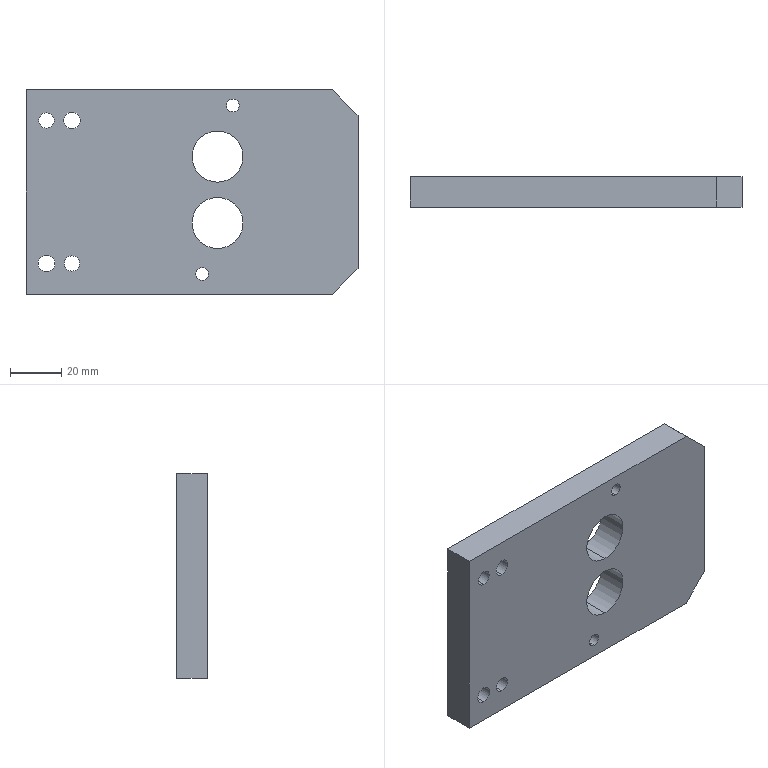Part | SolidWorks | features HoleWzd 3, 3DProfileFeature 2, Chamfer 1, Extrusion 1, ICE 1 | 1 solid | 30 faces | box 130 x 12 x 80 mm | volume 113262 mm3 | cylinder 20 | plane 10 | commonest cylinder face diameters 5 x4 6 x4 6.6 x4 11 x4 20 x4
STEP:
#1=CARTESIAN_POINT('',(81.,0.,-8.642));
#2=VERTEX_POINT('',#1);
#3=CARTESIAN_POINT('',(81.,0.,-3.642));
#4=VERTEX_POINT('',#3);
#5=CARTESIAN_POINT('',(81.,0.,-6.142));
#6=DIRECTION('',(0.,1.,0.));
#7=DIRECTION('',(0.,0.,1.));
#8=AXIS2_PLACEMENT_3D('',#5,#6,#7);
#9=CIRCLE('',#8,2.5);
#10=EDGE_CURVE('',#2,#4,#9,.T.);
#11=ORIENTED_EDGE('',*,*,#10,.F.);
#12=CARTESIAN_POINT('',(81.,12.,-8.642));
#13=VERTEX_POINT('',#12);
#14=CARTESIAN_POINT('',(81.,0.,-8.642));
#15=DIRECTION('',(0.,1.,0.));
#16=VECTOR('',#15,1000.);
#17=LINE('',#14,#16);
#18=EDGE_CURVE('',#2,#13,#17,.T.);
#19=ORIENTED_EDGE('',*,*,#18,.T.);
#20=CARTESIAN_POINT('',(81.,12.,-3.642));
#21=VERTEX_POINT('',#20);
#22=CARTESIAN_POINT('',(81.,12.,-6.142));
#23=DIRECTION('',(0.,1.,0.));
#24=DIRECTION('',(0.,0.,1.));
#25=AXIS2_PLACEMENT_3D('',#22,#23,#24);
#26=CIRCLE('',#25,2.5);
#27=EDGE_CURVE('',#13,#21,#26,.T.);
#28=ORIENTED_EDGE('',*,*,#27,.T.);
#29=CARTESIAN_POINT('',(81.,0.,-3.642));
#30=DIRECTION('',(0.,1.,0.));
#31=VECTOR('',#30,1000.);
#32=LINE('',#29,#31);
#33=EDGE_CURVE('',#4,#21,#32,.T.);
#34=ORIENTED_EDGE('',*,*,#33,.F.);
#35=EDGE_LOOP('',(#11,#19,#28,#34));
#36=FACE_OUTER_BOUND('',#35,.T.);
#37=CARTESIAN_POINT('',(81.,0.,-6.142));
#38=DIRECTION('',(0.,1.,0.));
#39=DIRECTION('',(0.,0.,1.));
#40=AXIS2_PLACEMENT_3D('',#37,#38,#39);
#41=CYLINDRICAL_SURFACE('',#40,2.5);
#42=ADVANCED_FACE('',(#36),#41,.F.);
#43=CARTESIAN_POINT('',(69.,0.,-74.642));
#44=VERTEX_POINT('',#43);
#45=CARTESIAN_POINT('',(69.,0.,-69.642));
#46=VERTEX_POINT('',#45);
#47=CARTESIAN_POINT('',(69.,0.,-72.142));
#48=DIRECTION('',(0.,1.,0.));
#49=DIRECTION('',(0.,0.,1.));
#50=AXIS2_PLACEMENT_3D('',#47,#48,#49);
#51=CIRCLE('',#50,2.5);
#52=EDGE_CURVE('',#44,#46,#51,.T.);
#53=ORIENTED_EDGE('',*,*,#52,.F.);
#54=CARTESIAN_POINT('',(69.,12.,-74.642));
#55=VERTEX_POINT('',#54);
#56=CARTESIAN_POINT('',(69.,0.,-74.642));
#57=DIRECTION('',(0.,1.,0.));
#58=VECTOR('',#57,1000.);
#59=LINE('',#56,#58);
#60=EDGE_CURVE('',#44,#55,#59,.T.);
#61=ORIENTED_EDGE('',*,*,#60,.T.);
#62=CARTESIAN_POINT('',(69.,12.,-69.642));
#63=VERTEX_POINT('',#62);
#64=CARTESIAN_POINT('',(69.,12.,-72.142));
#65=DIRECTION('',(0.,1.,0.));
#66=DIRECTION('',(0.,0.,1.));
#67=AXIS2_PLACEMENT_3D('',#64,#65,#66);
#68=CIRCLE('',#67,2.5);
#69=EDGE_CURVE('',#55,#63,#68,.T.);
#70=ORIENTED_EDGE('',*,*,#69,.T.);
#71=CARTESIAN_POINT('',(69.,0.,-69.642));
#72=DIRECTION('',(0.,1.,0.));
#73=VECTOR('',#72,1000.);
#74=LINE('',#71,#73);
#75=EDGE_CURVE('',#46,#63,#74,.T.);
#76=ORIENTED_EDGE('',*,*,#75,.F.);
#77=EDGE_LOOP('',(#53,#61,#70,#76));
#78=FACE_OUTER_BOUND('',#77,.T.);
#79=CARTESIAN_POINT('',(69.,0.,-72.142));
#80=DIRECTION('',(0.,1.,0.));
#81=DIRECTION('',(0.,0.,1.));
#82=AXIS2_PLACEMENT_3D('',#79,#80,#81);
#83=CYLINDRICAL_SURFACE('',#82,2.5);
#84=ADVANCED_FACE('',(#78),#83,.F.);
#85=CARTESIAN_POINT('',(75.,12.,-42.142));
#86=VERTEX_POINT('',#85);
#87=CARTESIAN_POINT('',(75.,12.,-62.142));
#88=VERTEX_POINT('',#87);
#89=CARTESIAN_POINT('',(75.,12.,-52.142));
#90=DIRECTION('',(0.,-1.,0.));
#91=DIRECTION('',(0.,0.,-1.));
#92=AXIS2_PLACEMENT_3D('',#89,#90,#91);
#93=CIRCLE('',#92,10.);
#94=EDGE_CURVE('',#86,#88,#93,.T.);
#95=ORIENTED_EDGE('',*,*,#94,.F.);
#96=CARTESIAN_POINT('',(75.,0.,-42.142));
#97=VERTEX_POINT('',#96);
#98=CARTESIAN_POINT('',(75.,0.,-42.142));
#99=DIRECTION('',(0.,-1.,0.));
#100=VECTOR('',#99,1000.);
#101=LINE('',#98,#100);
#102=EDGE_CURVE('',#86,#97,#101,.T.);
#103=ORIENTED_EDGE('',*,*,#102,.T.);
#104=CARTESIAN_POINT('',(75.,0.,-62.142));
#105=VERTEX_POINT('',#104);
#106=CARTESIAN_POINT('',(75.,0.,-52.142));
#107=DIRECTION('',(0.,-1.,0.));
#108=DIRECTION('',(0.,0.,-1.));
#109=AXIS2_PLACEMENT_3D('',#106,#107,#108);
#110=CIRCLE('',#109,10.);
#111=EDGE_CURVE('',#97,#105,#110,.T.);
#112=ORIENTED_EDGE('',*,*,#111,.T.);
#113=CARTESIAN_POINT('',(75.,0.,-62.142));
#114=DIRECTION('',(0.,-1.,0.));
#115=VECTOR('',#114,1000.);
#116=LINE('',#113,#115);
#117=EDGE_CURVE('',#88,#105,#116,.T.);
#118=ORIENTED_EDGE('',*,*,#117,.F.);
#119=EDGE_LOOP('',(#95,#103,#112,#118));
#120=FACE_OUTER_BOUND('',#119,.T.);
#121=CARTESIAN_POINT('',(75.,0.,-52.142));
#122=DIRECTION('',(0.,-1.,0.));
#123=DIRECTION('',(0.,0.,-1.));
#124=AXIS2_PLACEMENT_3D('',#121,#122,#123);
#125=CYLINDRICAL_SURFACE('',#124,10.);
#126=ADVANCED_FACE('',(#120),#125,.F.);
#127=CARTESIAN_POINT('',(75.,12.,-16.142));
#128=VERTEX_POINT('',#127);
#129=CARTESIAN_POINT('',(75.,12.,-36.142));
#130=VERTEX_POINT('',#129);
#131=CARTESIAN_POINT('',(75.,12.,-26.142));
#132=DIRECTION('',(0.,-1.,0.));
#133=DIRECTION('',(0.,0.,-1.));
#134=AXIS2_PLACEMENT_3D('',#131,#132,#133);
#135=CIRCLE('',#134,10.);
#136=EDGE_CURVE('',#128,#130,#135,.T.);
#137=ORIENTED_EDGE('',*,*,#136,.F.);
#138=CARTESIAN_POINT('',(75.,0.,-16.142));
#139=VERTEX_POINT('',#138);
#140=CARTESIAN_POINT('',(75.,0.,-16.142));
#141=DIRECTION('',(0.,-1.,0.));
#142=VECTOR('',#141,1000.);
#143=LINE('',#140,#142);
#144=EDGE_CURVE('',#128,#139,#143,.T.);
#145=ORIENTED_EDGE('',*,*,#144,.T.);
#146=CARTESIAN_POINT('',(75.,0.,-36.142));
#147=VERTEX_POINT('',#146);
#148=CARTESIAN_POINT('',(75.,0.,-26.142));
#149=DIRECTION('',(0.,-1.,0.));
#150=DIRECTION('',(0.,0.,-1.));
#151=AXIS2_PLACEMENT_3D('',#148,#149,#150);
#152=CIRCLE('',#151,10.);
#153=EDGE_CURVE('',#139,#147,#152,.T.);
#154=ORIENTED_EDGE('',*,*,#153,.T.);
#155=CARTESIAN_POINT('',(75.,0.,-36.142));
#156=DIRECTION('',(0.,-1.,0.));
#157=VECTOR('',#156,1000.);
#158=LINE('',#155,#157);
#159=EDGE_CURVE('',#130,#147,#158,.T.);
#160=ORIENTED_EDGE('',*,*,#159,.F.);
#161=EDGE_LOOP('',(#137,#145,#154,#160));
#162=FACE_OUTER_BOUND('',#161,.T.);
#163=CARTESIAN_POINT('',(75.,0.,-26.142));
#164=DIRECTION('',(0.,-1.,0.));
#165=DIRECTION('',(0.,0.,-1.));
#166=AXIS2_PLACEMENT_3D('',#163,#164,#165);
#167=CYLINDRICAL_SURFACE('',#166,10.);
#168=ADVANCED_FACE('',(#162),#167,.F.);
#169=CARTESIAN_POINT('',(18.,0.,-71.));
#170=VERTEX_POINT('',#169);
#171=CARTESIAN_POINT('',(18.,0.,-65.));
#172=VERTEX_POINT('',#171);
#173=CARTESIAN_POINT('',(18.,0.,-68.));
#174=DIRECTION('',(0.,1.,0.));
#175=DIRECTION('',(0.,0.,1.));
#176=AXIS2_PLACEMENT_3D('',#173,#174,#175);
#177=CIRCLE('',#176,3.);
#178=EDGE_CURVE('',#170,#172,#177,.T.);
#179=ORIENTED_EDGE('',*,*,#178,.F.);
#180=CARTESIAN_POINT('',(18.,12.,-71.));
#181=VERTEX_POINT('',#180);
#182=CARTESIAN_POINT('',(18.,12.,-71.));
#183=DIRECTION('',(0.,1.,0.));
#184=VECTOR('',#183,1000.);
#185=LINE('',#182,#184);
#186=EDGE_CURVE('',#170,#181,#185,.T.);
#187=ORIENTED_EDGE('',*,*,#186,.T.);
#188=CARTESIAN_POINT('',(18.,12.,-65.));
#189=VERTEX_POINT('',#188);
#190=CARTESIAN_POINT('',(18.,12.,-68.));
#191=DIRECTION('',(0.,1.,0.));
#192=DIRECTION('',(0.,0.,1.));
#193=AXIS2_PLACEMENT_3D('',#190,#191,#192);
#194=CIRCLE('',#193,3.);
#195=EDGE_CURVE('',#181,#189,#194,.T.);
#196=ORIENTED_EDGE('',*,*,#195,.T.);
#197=CARTESIAN_POINT('',(18.,12.,-65.));
#198=DIRECTION('',(0.,1.,0.));
#199=VECTOR('',#198,1000.);
#200=LINE('',#197,#199);
#201=EDGE_CURVE('',#172,#189,#200,.T.);
#202=ORIENTED_EDGE('',*,*,#201,.F.);
#203=EDGE_LOOP('',(#179,#187,#196,#202));
#204=FACE_OUTER_BOUND('',#203,.T.);
#205=CARTESIAN_POINT('',(18.,12.,-68.));
#206=DIRECTION('',(0.,1.,0.));
#207=DIRECTION('',(0.,0.,1.));
#208=AXIS2_PLACEMENT_3D('',#205,#206,#207);
#209=CYLINDRICAL_SURFACE('',#208,3.);
#210=ADVANCED_FACE('',(#204),#209,.F.);
#211=CARTESIAN_POINT('',(8.,0.,-15.));
#212=VERTEX_POINT('',#211);
#213=CARTESIAN_POINT('',(8.,0.,-9.));
#214=VERTEX_POINT('',#213);
#215=CARTESIAN_POINT('',(8.,0.,-12.));
#216=DIRECTION('',(0.,1.,0.));
#217=DIRECTION('',(0.,0.,1.));
#218=AXIS2_PLACEMENT_3D('',#215,#216,#217);
#219=CIRCLE('',#218,3.);
#220=EDGE_CURVE('',#212,#214,#219,.T.);
#221=ORIENTED_EDGE('',*,*,#220,.F.);
#222=CARTESIAN_POINT('',(8.,12.,-15.));
#223=VERTEX_POINT('',#222);
#224=CARTESIAN_POINT('',(8.,12.,-15.));
#225=DIRECTION('',(0.,1.,0.));
#226=VECTOR('',#225,1000.);
#227=LINE('',#224,#226);
#228=EDGE_CURVE('',#212,#223,#227,.T.);
#229=ORIENTED_EDGE('',*,*,#228,.T.);
#230=CARTESIAN_POINT('',(8.,12.,-9.));
#231=VERTEX_POINT('',#230);
#232=CARTESIAN_POINT('',(8.,12.,-12.));
#233=DIRECTION('',(0.,1.,0.));
#234=DIRECTION('',(0.,0.,1.));
#235=AXIS2_PLACEMENT_3D('',#232,#233,#234);
#236=CIRCLE('',#235,3.);
#237=EDGE_CURVE('',#223,#231,#236,.T.);
#238=ORIENTED_EDGE('',*,*,#237,.T.);
#239=CARTESIAN_POINT('',(8.,12.,-9.));
#240=DIRECTION('',(0.,1.,0.));
#241=VECTOR('',#240,1000.);
#242=LINE('',#239,#241);
#243=EDGE_CURVE('',#214,#231,#242,.T.);
#244=ORIENTED_EDGE('',*,*,#243,.F.);
#245=EDGE_LOOP('',(#221,#229,#238,#244));
#246=FACE_OUTER_BOUND('',#245,.T.);
#247=CARTESIAN_POINT('',(8.,12.,-12.));
#248=DIRECTION('',(0.,1.,0.));
#249=DIRECTION('',(0.,0.,1.));
#250=AXIS2_PLACEMENT_3D('',#247,#248,#249);
#251=CYLINDRICAL_SURFACE('',#250,3.);
#252=ADVANCED_FACE('',(#246),#251,.F.);
#253=CARTESIAN_POINT('',(8.,5.2,-73.5));
#254=VERTEX_POINT('',#253);
#255=CARTESIAN_POINT('',(8.,5.2,-62.5));
#256=VERTEX_POINT('',#255);
#257=CARTESIAN_POINT('',(8.,5.2,-68.));
#258=DIRECTION('',(0.,1.,0.));
#259=DIRECTION('',(0.,0.,1.));
#260=AXIS2_PLACEMENT_3D('',#257,#258,#259);
#261=CIRCLE('',#260,5.5);
#262=EDGE_CURVE('',#254,#256,#261,.T.);
#263=ORIENTED_EDGE('',*,*,#262,.F.);
#264=CARTESIAN_POINT('',(8.,12.,-73.5));
#265=VERTEX_POINT('',#264);
#266=CARTESIAN_POINT('',(8.,12.,-73.5));
#267=DIRECTION('',(0.,1.,0.));
#268=VECTOR('',#267,1000.);
#269=LINE('',#266,#268);
#270=EDGE_CURVE('',#254,#265,#269,.T.);
#271=ORIENTED_EDGE('',*,*,#270,.T.);
#272=CARTESIAN_POINT('',(8.,12.,-62.5));
#273=VERTEX_POINT('',#272);
#274=CARTESIAN_POINT('',(8.,12.,-68.));
#275=DIRECTION('',(0.,1.,0.));
#276=DIRECTION('',(0.,0.,1.));
#277=AXIS2_PLACEMENT_3D('',#274,#275,#276);
#278=CIRCLE('',#277,5.5);
#279=EDGE_CURVE('',#265,#273,#278,.T.);
#280=ORIENTED_EDGE('',*,*,#279,.T.);
#281=CARTESIAN_POINT('',(8.,12.,-62.5));
#282=DIRECTION('',(0.,1.,0.));
#283=VECTOR('',#282,1000.);
#284=LINE('',#281,#283);
#285=EDGE_CURVE('',#256,#273,#284,.T.);
#286=ORIENTED_EDGE('',*,*,#285,.F.);
#287=EDGE_LOOP('',(#263,#271,#280,#286));
#288=FACE_OUTER_BOUND('',#287,.T.);
#289=CARTESIAN_POINT('',(8.,12.,-68.));
#290=DIRECTION('',(0.,1.,0.));
#291=DIRECTION('',(0.,0.,1.));
#292=AXIS2_PLACEMENT_3D('',#289,#290,#291);
#293=CYLINDRICAL_SURFACE('',#292,5.5);
#294=ADVANCED_FACE('',(#288),#293,.F.);
#295=CARTESIAN_POINT('',(8.,0.,-71.3));
#296=VERTEX_POINT('',#295);
#297=CARTESIAN_POINT('',(8.,0.,-64.7));
#298=VERTEX_POINT('',#297);
#299=CARTESIAN_POINT('',(8.,0.,-68.));
#300=DIRECTION('',(0.,1.,0.));
#301=DIRECTION('',(0.,0.,1.));
#302=AXIS2_PLACEMENT_3D('',#299,#300,#301);
#303=CIRCLE('',#302,3.3);
#304=EDGE_CURVE('',#296,#298,#303,.T.);
#305=ORIENTED_EDGE('',*,*,#304,.F.);
#306=CARTESIAN_POINT('',(8.,5.2,-71.3));
#307=VERTEX_POINT('',#306);
#308=CARTESIAN_POINT('',(8.,12.,-71.3));
#309=DIRECTION('',(0.,1.,0.));
#310=VECTOR('',#309,1000.);
#311=LINE('',#308,#310);
#312=EDGE_CURVE('',#296,#307,#311,.T.);
#313=ORIENTED_EDGE('',*,*,#312,.T.);
#314=CARTESIAN_POINT('',(8.,5.2,-64.7));
#315=VERTEX_POINT('',#314);
#316=CARTESIAN_POINT('',(8.,5.2,-68.));
#317=DIRECTION('',(0.,1.,0.));
#318=DIRECTION('',(0.,0.,1.));
#319=AXIS2_PLACEMENT_3D('',#316,#317,#318);
#320=CIRCLE('',#319,3.3);
#321=EDGE_CURVE('',#307,#315,#320,.T.);
#322=ORIENTED_EDGE('',*,*,#321,.T.);
#323=CARTESIAN_POINT('',(8.,12.,-64.7));
#324=DIRECTION('',(0.,1.,0.));
#325=VECTOR('',#324,1000.);
#326=LINE('',#323,#325);
#327=EDGE_CURVE('',#298,#315,#326,.T.);
#328=ORIENTED_EDGE('',*,*,#327,.F.);
#329=EDGE_LOOP('',(#305,#313,#322,#328));
#330=FACE_OUTER_BOUND('',#329,.T.);
#331=CARTESIAN_POINT('',(8.,12.,-68.));
#332=DIRECTION('',(0.,1.,0.));
#333=DIRECTION('',(0.,0.,1.));
#334=AXIS2_PLACEMENT_3D('',#331,#332,#333);
#335=CYLINDRICAL_SURFACE('',#334,3.3);
#336=ADVANCED_FACE('',(#330),#335,.F.);
#337=CARTESIAN_POINT('',(18.,5.2,-17.5));
#338=VERTEX_POINT('',#337);
#339=CARTESIAN_POINT('',(18.,5.2,-6.5));
#340=VERTEX_POINT('',#339);
#341=CARTESIAN_POINT('',(18.,5.2,-12.));
#342=DIRECTION('',(0.,1.,0.));
#343=DIRECTION('',(0.,0.,1.));
#344=AXIS2_PLACEMENT_3D('',#341,#342,#343);
#345=CIRCLE('',#344,5.5);
#346=EDGE_CURVE('',#338,#340,#345,.T.);
#347=ORIENTED_EDGE('',*,*,#346,.F.);
#348=CARTESIAN_POINT('',(18.,12.,-17.5));
#349=VERTEX_POINT('',#348);
#350=CARTESIAN_POINT('',(18.,12.,-17.5));
#351=DIRECTION('',(0.,1.,0.));
#352=VECTOR('',#351,1000.);
#353=LINE('',#350,#352);
#354=EDGE_CURVE('',#338,#349,#353,.T.);
#355=ORIENTED_EDGE('',*,*,#354,.T.);
#356=CARTESIAN_POINT('',(18.,12.,-6.5));
#357=VERTEX_POINT('',#356);
#358=CARTESIAN_POINT('',(18.,12.,-12.));
#359=DIRECTION('',(0.,1.,0.));
#360=DIRECTION('',(0.,0.,1.));
#361=AXIS2_PLACEMENT_3D('',#358,#359,#360);
#362=CIRCLE('',#361,5.5);
#363=EDGE_CURVE('',#349,#357,#362,.T.);
#364=ORIENTED_EDGE('',*,*,#363,.T.);
#365=CARTESIAN_POINT('',(18.,12.,-6.5));
#366=DIRECTION('',(0.,1.,0.));
#367=VECTOR('',#366,1000.);
#368=LINE('',#365,#367);
#369=EDGE_CURVE('',#340,#357,#368,.T.);
#370=ORIENTED_EDGE('',*,*,#369,.F.);
#371=EDGE_LOOP('',(#347,#355,#364,#370));
#372=FACE_OUTER_BOUND('',#371,.T.);
#373=CARTESIAN_POINT('',(18.,12.,-12.));
#374=DIRECTION('',(0.,1.,0.));
#375=DIRECTION('',(0.,0.,1.));
#376=AXIS2_PLACEMENT_3D('',#373,#374,#375);
#377=CYLINDRICAL_SURFACE('',#376,5.5);
#378=ADVANCED_FACE('',(#372),#377,.F.);
#379=CARTESIAN_POINT('',(18.,0.,-15.3));
#380=VERTEX_POINT('',#379);
#381=CARTESIAN_POINT('',(18.,0.,-8.7));
#382=VERTEX_POINT('',#381);
#383=CARTESIAN_POINT('',(18.,0.,-12.));
#384=DIRECTION('',(0.,1.,0.));
#385=DIRECTION('',(0.,0.,1.));
#386=AXIS2_PLACEMENT_3D('',#383,#384,#385);
#387=CIRCLE('',#386,3.3);
#388=EDGE_CURVE('',#380,#382,#387,.T.);
#389=ORIENTED_EDGE('',*,*,#388,.F.);
#390=CARTESIAN_POINT('',(18.,5.2,-15.3));
#391=VERTEX_POINT('',#390);
#392=CARTESIAN_POINT('',(18.,12.,-15.3));
#393=DIRECTION('',(0.,1.,0.));
#394=VECTOR('',#393,1000.);
#395=LINE('',#392,#394);
#396=EDGE_CURVE('',#380,#391,#395,.T.);
#397=ORIENTED_EDGE('',*,*,#396,.T.);
#398=CARTESIAN_POINT('',(18.,5.2,-8.7));
#399=VERTEX_POINT('',#398);
#400=CARTESIAN_POINT('',(18.,5.2,-12.));
#401=DIRECTION('',(0.,1.,0.));
#402=DIRECTION('',(0.,0.,1.));
#403=AXIS2_PLACEMENT_3D('',#400,#401,#402);
#404=CIRCLE('',#403,3.3);
#405=EDGE_CURVE('',#391,#399,#404,.T.);
#406=ORIENTED_EDGE('',*,*,#405,.T.);
#407=CARTESIAN_POINT('',(18.,12.,-8.7));
#408=DIRECTION('',(0.,1.,0.));
#409=VECTOR('',#408,1000.);
#410=LINE('',#407,#409);
#411=EDGE_CURVE('',#382,#399,#410,.T.);
#412=ORIENTED_EDGE('',*,*,#411,.F.);
#413=EDGE_LOOP('',(#389,#397,#406,#412));
#414=FACE_OUTER_BOUND('',#413,.T.);
#415=CARTESIAN_POINT('',(18.,12.,-12.));
#416=DIRECTION('',(0.,1.,0.));
#417=DIRECTION('',(0.,0.,1.));
#418=AXIS2_PLACEMENT_3D('',#415,#416,#417);
#419=CYLINDRICAL_SURFACE('',#418,3.3);
#420=ADVANCED_FACE('',(#414),#419,.F.);
#421=CARTESIAN_POINT('',(81.,0.,-6.142));
#422=DIRECTION('',(0.,1.,0.));
#423=DIRECTION('',(0.,0.,1.));
#424=AXIS2_PLACEMENT_3D('',#421,#422,#423);
#425=CIRCLE('',#424,2.5);
#426=EDGE_CURVE('',#4,#2,#425,.T.);
#427=ORIENTED_EDGE('',*,*,#426,.T.);
#428=ORIENTED_EDGE('',*,*,#10,.T.);
#429=EDGE_LOOP('',(#427,#428));
#430=FACE_BOUND('',#429,.T.);
#431=CARTESIAN_POINT('',(69.,0.,-72.142));
#432=DIRECTION('',(0.,1.,0.));
#433=DIRECTION('',(0.,0.,1.));
#434=AXIS2_PLACEMENT_3D('',#431,#432,#433);
#435=CIRCLE('',#434,2.5);
#436=EDGE_CURVE('',#46,#44,#435,.T.);
#437=ORIENTED_EDGE('',*,*,#436,.T.);
#438=ORIENTED_EDGE('',*,*,#52,.T.);
#439=EDGE_LOOP('',(#437,#438));
#440=FACE_BOUND('',#439,.T.);
#441=CARTESIAN_POINT('',(75.,0.,-52.142));
#442=DIRECTION('',(0.,-1.,0.));
#443=DIRECTION('',(0.,0.,-1.));
#444=AXIS2_PLACEMENT_3D('',#441,#442,#443);
#445=CIRCLE('',#444,10.);
#446=EDGE_CURVE('',#105,#97,#445,.T.);
#447=ORIENTED_EDGE('',*,*,#446,.F.);
#448=ORIENTED_EDGE('',*,*,#111,.F.);
#449=EDGE_LOOP('',(#447,#448));
#450=FACE_BOUND('',#449,.T.);
#451=CARTESIAN_POINT('',(75.,0.,-26.142));
#452=DIRECTION('',(0.,-1.,0.));
#453=DIRECTION('',(0.,0.,-1.));
#454=AXIS2_PLACEMENT_3D('',#451,#452,#453);
#455=CIRCLE('',#454,10.);
#456=EDGE_CURVE('',#147,#139,#455,.T.);
#457=ORIENTED_EDGE('',*,*,#456,.F.);
#458=ORIENTED_EDGE('',*,*,#153,.F.);
#459=EDGE_LOOP('',(#457,#458));
#460=FACE_BOUND('',#459,.T.);
#461=CARTESIAN_POINT('',(18.,0.,-68.));
#462=DIRECTION('',(0.,1.,0.));
#463=DIRECTION('',(0.,0.,1.));
#464=AXIS2_PLACEMENT_3D('',#461,#462,#463);
#465=CIRCLE('',#464,3.);
#466=EDGE_CURVE('',#172,#170,#465,.T.);
#467=ORIENTED_EDGE('',*,*,#466,.T.);
#468=ORIENTED_EDGE('',*,*,#178,.T.);
#469=EDGE_LOOP('',(#467,#468));
#470=FACE_BOUND('',#469,.T.);
#471=CARTESIAN_POINT('',(120.,0.,-80.));
#472=VERTEX_POINT('',#471);
#473=CARTESIAN_POINT('',(0.,0.,-80.));
#474=VERTEX_POINT('',#473);
#475=CARTESIAN_POINT('',(0.,0.,-80.));
#476=DIRECTION('',(-1.,0.,0.));
#477=VECTOR('',#476,1000.);
#478=LINE('',#475,#477);
#479=EDGE_CURVE('',#472,#474,#478,.T.);
#480=ORIENTED_EDGE('',*,*,#479,.F.);
#481=CARTESIAN_POINT('',(130.,0.,-70.));
#482=VERTEX_POINT('',#481);
#483=CARTESIAN_POINT('',(100.,0.,-100.));
#484=DIRECTION('',(0.7071,0.,0.7071));
#485=VECTOR('',#484,1000.);
#486=LINE('',#483,#485);
#487=EDGE_CURVE('',#472,#482,#486,.T.);
#488=ORIENTED_EDGE('',*,*,#487,.T.);
#489=CARTESIAN_POINT('',(130.,0.,-10.));
#490=VERTEX_POINT('',#489);
#491=CARTESIAN_POINT('',(130.,0.,0.));
#492=DIRECTION('',(0.,0.,-1.));
#493=VECTOR('',#492,1000.);
#494=LINE('',#491,#493);
#495=EDGE_CURVE('',#490,#482,#494,.T.);
#496=ORIENTED_EDGE('',*,*,#495,.F.);
#497=CARTESIAN_POINT('',(120.,0.,0.));
#498=VERTEX_POINT('',#497);
#499=CARTESIAN_POINT('',(60.,0.,60.));
#500=DIRECTION('',(-0.7071,0.,0.7071));
#501=VECTOR('',#500,1000.);
#502=LINE('',#499,#501);
#503=EDGE_CURVE('',#490,#498,#502,.T.);
#504=ORIENTED_EDGE('',*,*,#503,.T.);
#505=CARTESIAN_POINT('',(0.,0.,0.));
#506=VERTEX_POINT('',#505);
#507=CARTESIAN_POINT('',(0.,0.,0.));
#508=DIRECTION('',(1.,0.,0.));
#509=VECTOR('',#508,1000.);
#510=LINE('',#507,#509);
#511=EDGE_CURVE('',#506,#498,#510,.T.);
#512=ORIENTED_EDGE('',*,*,#511,.F.);
#513=CARTESIAN_POINT('',(0.,0.,0.));
#514=DIRECTION('',(0.,0.,1.));
#515=VECTOR('',#514,1000.);
#516=LINE('',#513,#515);
#517=EDGE_CURVE('',#474,#506,#516,.T.);
#518=ORIENTED_EDGE('',*,*,#517,.F.);
#519=EDGE_LOOP('',(#480,#488,#496,#504,#512,#518));
#520=FACE_OUTER_BOUND('',#519,.T.);
#521=CARTESIAN_POINT('',(18.,0.,-12.));
#522=DIRECTION('',(0.,1.,0.));
#523=DIRECTION('',(0.,0.,1.));
#524=AXIS2_PLACEMENT_3D('',#521,#522,#523);
#525=CIRCLE('',#524,3.3);
#526=EDGE_CURVE('',#382,#380,#525,.T.);
#527=ORIENTED_EDGE('',*,*,#526,.T.);
#528=ORIENTED_EDGE('',*,*,#388,.T.);
#529=EDGE_LOOP('',(#527,#528));
#530=FACE_BOUND('',#529,.T.);
#531=CARTESIAN_POINT('',(8.,0.,-68.));
#532=DIRECTION('',(0.,1.,0.));
#533=DIRECTION('',(0.,0.,1.));
#534=AXIS2_PLACEMENT_3D('',#531,#532,#533);
#535=CIRCLE('',#534,3.3);
#536=EDGE_CURVE('',#298,#296,#535,.T.);
#537=ORIENTED_EDGE('',*,*,#536,.T.);
#538=ORIENTED_EDGE('',*,*,#304,.T.);
#539=EDGE_LOOP('',(#537,#538));
#540=FACE_BOUND('',#539,.T.);
#541=CARTESIAN_POINT('',(8.,0.,-12.));
#542=DIRECTION('',(0.,1.,0.));
#543=DIRECTION('',(0.,0.,1.));
#544=AXIS2_PLACEMENT_3D('',#541,#542,#543);
#545=CIRCLE('',#544,3.);
#546=EDGE_CURVE('',#214,#212,#545,.T.);
#547=ORIENTED_EDGE('',*,*,#546,.T.);
#548=ORIENTED_EDGE('',*,*,#220,.T.);
#549=EDGE_LOOP('',(#547,#548));
#550=FACE_BOUND('',#549,.T.);
#551=CARTESIAN_POINT('',(0.,0.,0.));
#552=DIRECTION('',(0.,-1.,0.));
#553=DIRECTION('',(0.,0.,-1.));
#554=AXIS2_PLACEMENT_3D('',#551,#552,#553);
#555=PLANE('',#554);
#556=ADVANCED_FACE('',(#430,#440,#450,#460,#470,#520,#530,#540,#550),#555,.T.);
#557=ORIENTED_EDGE('',*,*,#517,.T.);
#558=CARTESIAN_POINT('',(0.,12.,0.));
#559=VERTEX_POINT('',#558);
#560=CARTESIAN_POINT('',(0.,12.,0.));
#561=DIRECTION('',(0.,-1.,0.));
#562=VECTOR('',#561,1000.);
#563=LINE('',#560,#562);
#564=EDGE_CURVE('',#559,#506,#563,.T.);
#565=ORIENTED_EDGE('',*,*,#564,.F.);
#566=CARTESIAN_POINT('',(0.,12.,-80.));
#567=VERTEX_POINT('',#566);
#568=CARTESIAN_POINT('',(0.,12.,0.));
#569=DIRECTION('',(0.,0.,1.));
#570=VECTOR('',#569,1000.);
#571=LINE('',#568,#570);
#572=EDGE_CURVE('',#567,#559,#571,.T.);
#573=ORIENTED_EDGE('',*,*,#572,.F.);
#574=CARTESIAN_POINT('',(0.,12.,-80.));
#575=DIRECTION('',(0.,-1.,0.));
#576=VECTOR('',#575,1000.);
#577=LINE('',#574,#576);
#578=EDGE_CURVE('',#567,#474,#577,.T.);
#579=ORIENTED_EDGE('',*,*,#578,.T.);
#580=EDGE_LOOP('',(#557,#565,#573,#579));
#581=FACE_OUTER_BOUND('',#580,.T.);
#582=CARTESIAN_POINT('',(0.,12.,0.));
#583=DIRECTION('',(1.,0.,0.));
#584=DIRECTION('',(0.,0.,-1.));
#585=AXIS2_PLACEMENT_3D('',#582,#583,#584);
#586=PLANE('',#585);
#587=ADVANCED_FACE('',(#581),#586,.F.);
#588=ORIENTED_EDGE('',*,*,#511,.T.);
#589=CARTESIAN_POINT('',(120.,12.,0.));
#590=VERTEX_POINT('',#589);
#591=CARTESIAN_POINT('',(120.,12.,0.));
#592=DIRECTION('',(0.,1.,0.));
#593=VECTOR('',#592,1000.);
#594=LINE('',#591,#593);
#595=EDGE_CURVE('',#498,#590,#594,.T.);
#596=ORIENTED_EDGE('',*,*,#595,.T.);
#597=CARTESIAN_POINT('',(0.,12.,0.));
#598=DIRECTION('',(1.,0.,0.));
#599=VECTOR('',#598,1000.);
#600=LINE('',#597,#599);
#601=EDGE_CURVE('',#559,#590,#600,.T.);
#602=ORIENTED_EDGE('',*,*,#601,.F.);
#603=ORIENTED_EDGE('',*,*,#564,.T.);
#604=EDGE_LOOP('',(#588,#596,#602,#603));
#605=FACE_OUTER_BOUND('',#604,.T.);
#606=CARTESIAN_POINT('',(0.,12.,0.));
#607=DIRECTION('',(0.,0.,-1.));
#608=DIRECTION('',(-1.,0.,0.));
#609=AXIS2_PLACEMENT_3D('',#606,#607,#608);
#610=PLANE('',#609);
#611=ADVANCED_FACE('',(#605),#610,.F.);
#612=ORIENTED_EDGE('',*,*,#495,.T.);
#613=CARTESIAN_POINT('',(130.,12.,-70.));
#614=VERTEX_POINT('',#613);
#615=CARTESIAN_POINT('',(130.,12.,-70.));
#616=DIRECTION('',(0.,1.,0.));
#617=VECTOR('',#616,1000.);
#618=LINE('',#615,#617);
#619=EDGE_CURVE('',#482,#614,#618,.T.);
#620=ORIENTED_EDGE('',*,*,#619,.T.);
#621=CARTESIAN_POINT('',(130.,12.,-10.));
#622=VERTEX_POINT('',#621);
#623=CARTESIAN_POINT('',(130.,12.,0.));
#624=DIRECTION('',(0.,0.,-1.));
#625=VECTOR('',#624,1000.);
#626=LINE('',#623,#625);
#627=EDGE_CURVE('',#622,#614,#626,.T.);
#628=ORIENTED_EDGE('',*,*,#627,.F.);
#629=CARTESIAN_POINT('',(130.,12.,-10.));
#630=DIRECTION('',(0.,-1.,0.));
#631=VECTOR('',#630,1000.);
#632=LINE('',#629,#631);
#633=EDGE_CURVE('',#622,#490,#632,.T.);
#634=ORIENTED_EDGE('',*,*,#633,.T.);
#635=EDGE_LOOP('',(#612,#620,#628,#634));
#636=FACE_OUTER_BOUND('',#635,.T.);
#637=CARTESIAN_POINT('',(130.,12.,0.));
#638=DIRECTION('',(-1.,0.,0.));
#639=DIRECTION('',(0.,0.,1.));
#640=AXIS2_PLACEMENT_3D('',#637,#638,#639);
#641=PLANE('',#640);
#642=ADVANCED_FACE('',(#636),#641,.F.);
#643=CARTESIAN_POINT('',(120.,12.,-80.));
#644=VERTEX_POINT('',#643);
#645=CARTESIAN_POINT('',(0.,12.,-80.));
#646=DIRECTION('',(-1.,0.,0.));
#647=VECTOR('',#646,1000.);
#648=LINE('',#645,#647);
#649=EDGE_CURVE('',#644,#567,#648,.T.);
#650=ORIENTED_EDGE('',*,*,#649,.F.);
#651=CARTESIAN_POINT('',(120.,12.,-80.));
#652=DIRECTION('',(0.,-1.,0.));
#653=VECTOR('',#652,1000.);
#654=LINE('',#651,#653);
#655=EDGE_CURVE('',#644,#472,#654,.T.);
#656=ORIENTED_EDGE('',*,*,#655,.T.);
#657=ORIENTED_EDGE('',*,*,#479,.T.);
#658=ORIENTED_EDGE('',*,*,#578,.F.);
#659=EDGE_LOOP('',(#650,#656,#657,#658));
#660=FACE_OUTER_BOUND('',#659,.T.);
#661=CARTESIAN_POINT('',(0.,12.,-80.));
#662=DIRECTION('',(0.,0.,1.));
#663=DIRECTION('',(1.,0.,0.));
#664=AXIS2_PLACEMENT_3D('',#661,#662,#663);
#665=PLANE('',#664);
#666=ADVANCED_FACE('',(#660),#665,.F.);
#667=CARTESIAN_POINT('',(81.,12.,-6.142));
#668=DIRECTION('',(0.,1.,0.));
#669=DIRECTION('',(0.,0.,1.));
#670=AXIS2_PLACEMENT_3D('',#667,#668,#669);
#671=CIRCLE('',#670,2.5);
#672=EDGE_CURVE('',#21,#13,#671,.T.);
#673=ORIENTED_EDGE('',*,*,#672,.F.);
#674=ORIENTED_EDGE('',*,*,#27,.F.);
#675=EDGE_LOOP('',(#673,#674));
#676=FACE_BOUND('',#675,.T.);
#677=CARTESIAN_POINT('',(69.,12.,-72.142));
#678=DIRECTION('',(0.,1.,0.));
#679=DIRECTION('',(0.,0.,1.));
#680=AXIS2_PLACEMENT_3D('',#677,#678,#679);
#681=CIRCLE('',#680,2.5);
#682=EDGE_CURVE('',#63,#55,#681,.T.);
#683=ORIENTED_EDGE('',*,*,#682,.F.);
#684=ORIENTED_EDGE('',*,*,#69,.F.);
#685=EDGE_LOOP('',(#683,#684));
#686=FACE_BOUND('',#685,.T.);
#687=CARTESIAN_POINT('',(75.,12.,-52.142));
#688=DIRECTION('',(0.,-1.,0.));
#689=DIRECTION('',(0.,0.,-1.));
#690=AXIS2_PLACEMENT_3D('',#687,#688,#689);
#691=CIRCLE('',#690,10.);
#692=EDGE_CURVE('',#88,#86,#691,.T.);
#693=ORIENTED_EDGE('',*,*,#692,.T.);
#694=ORIENTED_EDGE('',*,*,#94,.T.);
#695=EDGE_LOOP('',(#693,#694));
#696=FACE_BOUND('',#695,.T.);
#697=CARTESIAN_POINT('',(75.,12.,-26.142));
#698=DIRECTION('',(0.,-1.,0.));
#699=DIRECTION('',(0.,0.,-1.));
#700=AXIS2_PLACEMENT_3D('',#697,#698,#699);
#701=CIRCLE('',#700,10.);
#702=EDGE_CURVE('',#130,#128,#701,.T.);
#703=ORIENTED_EDGE('',*,*,#702,.T.);
#704=ORIENTED_EDGE('',*,*,#136,.T.);
#705=EDGE_LOOP('',(#703,#704));
#706=FACE_BOUND('',#705,.T.);
#707=CARTESIAN_POINT('',(18.,12.,-68.));
#708=DIRECTION('',(0.,1.,0.));
#709=DIRECTION('',(0.,0.,1.));
#710=AXIS2_PLACEMENT_3D('',#707,#708,#709);
#711=CIRCLE('',#710,3.);
#712=EDGE_CURVE('',#189,#181,#711,.T.);
#713=ORIENTED_EDGE('',*,*,#712,.F.);
#714=ORIENTED_EDGE('',*,*,#195,.F.);
#715=EDGE_LOOP('',(#713,#714));
#716=FACE_BOUND('',#715,.T.);
#717=CARTESIAN_POINT('',(8.,12.,-12.));
#718=DIRECTION('',(0.,1.,0.));
#719=DIRECTION('',(0.,0.,1.));
#720=AXIS2_PLACEMENT_3D('',#717,#718,#719);
#721=CIRCLE('',#720,3.);
#722=EDGE_CURVE('',#231,#223,#721,.T.);
#723=ORIENTED_EDGE('',*,*,#722,.F.);
#724=ORIENTED_EDGE('',*,*,#237,.F.);
#725=EDGE_LOOP('',(#723,#724));
#726=FACE_BOUND('',#725,.T.);
#727=CARTESIAN_POINT('',(8.,12.,-68.));
#728=DIRECTION('',(0.,1.,0.));
#729=DIRECTION('',(0.,0.,1.));
#730=AXIS2_PLACEMENT_3D('',#727,#728,#729);
#731=CIRCLE('',#730,5.5);
#732=EDGE_CURVE('',#273,#265,#731,.T.);
#733=ORIENTED_EDGE('',*,*,#732,.F.);
#734=ORIENTED_EDGE('',*,*,#279,.F.);
#735=EDGE_LOOP('',(#733,#734));
#736=FACE_BOUND('',#735,.T.);
#737=CARTESIAN_POINT('',(18.,12.,-12.));
#738=DIRECTION('',(0.,1.,0.));
#739=DIRECTION('',(0.,0.,1.));
#740=AXIS2_PLACEMENT_3D('',#737,#738,#739);
#741=CIRCLE('',#740,5.5);
#742=EDGE_CURVE('',#357,#349,#741,.T.);
#743=ORIENTED_EDGE('',*,*,#742,.F.);
#744=ORIENTED_EDGE('',*,*,#363,.F.);
#745=EDGE_LOOP('',(#743,#744));
#746=FACE_BOUND('',#745,.T.);
#747=ORIENTED_EDGE('',*,*,#627,.T.);
#748=CARTESIAN_POINT('',(120.,12.,-80.));
#749=DIRECTION('',(-0.7071,0.,-0.7071));
#750=VECTOR('',#749,1000.);
#751=LINE('',#748,#750);
#752=EDGE_CURVE('',#614,#644,#751,.T.);
#753=ORIENTED_EDGE('',*,*,#752,.T.);
#754=ORIENTED_EDGE('',*,*,#649,.T.);
#755=ORIENTED_EDGE('',*,*,#572,.T.);
#756=ORIENTED_EDGE('',*,*,#601,.T.);
#757=CARTESIAN_POINT('',(130.,12.,-10.));
#758=DIRECTION('',(0.7071,0.,-0.7071));
#759=VECTOR('',#758,1000.);
#760=LINE('',#757,#759);
#761=EDGE_CURVE('',#590,#622,#760,.T.);
#762=ORIENTED_EDGE('',*,*,#761,.T.);
#763=EDGE_LOOP('',(#747,#753,#754,#755,#756,#762));
#764=FACE_OUTER_BOUND('',#763,.T.);
#765=CARTESIAN_POINT('',(0.,12.,0.));
#766=DIRECTION('',(0.,-1.,0.));
#767=DIRECTION('',(0.,0.,-1.));
#768=AXIS2_PLACEMENT_3D('',#765,#766,#767);
#769=PLANE('',#768);
#770=ADVANCED_FACE('',(#676,#686,#696,#706,#716,#726,#736,#746,#764),#769,.F.);
#771=ORIENTED_EDGE('',*,*,#752,.F.);
#772=ORIENTED_EDGE('',*,*,#619,.F.);
#773=ORIENTED_EDGE('',*,*,#487,.F.);
#774=ORIENTED_EDGE('',*,*,#655,.F.);
#775=EDGE_LOOP('',(#771,#772,#773,#774));
#776=FACE_OUTER_BOUND('',#775,.T.);
#777=CARTESIAN_POINT('',(120.,12.,-80.));
#778=DIRECTION('',(-0.7071,0.,0.7071));
#779=DIRECTION('',(0.,-1.,0.));
#780=AXIS2_PLACEMENT_3D('',#777,#778,#779);
#781=PLANE('',#780);
#782=ADVANCED_FACE('',(#776),#781,.F.);
#783=ORIENTED_EDGE('',*,*,#761,.F.);
#784=ORIENTED_EDGE('',*,*,#595,.F.);
#785=ORIENTED_EDGE('',*,*,#503,.F.);
#786=ORIENTED_EDGE('',*,*,#633,.F.);
#787=EDGE_LOOP('',(#783,#784,#785,#786));
#788=FACE_OUTER_BOUND('',#787,.T.);
#789=CARTESIAN_POINT('',(130.,12.,-10.));
#790=DIRECTION('',(-0.7071,0.,-0.7071));
#791=DIRECTION('',(0.,-1.,0.));
#792=AXIS2_PLACEMENT_3D('',#789,#790,#791);
#793=PLANE('',#792);
#794=ADVANCED_FACE('',(#788),#793,.F.);
#795=ORIENTED_EDGE('',*,*,#396,.F.);
#796=ORIENTED_EDGE('',*,*,#526,.F.);
#797=ORIENTED_EDGE('',*,*,#411,.T.);
#798=CARTESIAN_POINT('',(18.,5.2,-12.));
#799=DIRECTION('',(0.,1.,0.));
#800=DIRECTION('',(0.,0.,1.));
#801=AXIS2_PLACEMENT_3D('',#798,#799,#800);
#802=CIRCLE('',#801,3.3);
#803=EDGE_CURVE('',#399,#391,#802,.T.);
#804=ORIENTED_EDGE('',*,*,#803,.T.);
#805=EDGE_LOOP('',(#795,#796,#797,#804));
#806=FACE_OUTER_BOUND('',#805,.T.);
#807=CARTESIAN_POINT('',(18.,12.,-12.));
#808=DIRECTION('',(0.,1.,0.));
#809=DIRECTION('',(0.,0.,1.));
#810=AXIS2_PLACEMENT_3D('',#807,#808,#809);
#811=CYLINDRICAL_SURFACE('',#810,3.3);
#812=ADVANCED_FACE('',(#806),#811,.F.);
#813=ORIENTED_EDGE('',*,*,#803,.F.);
#814=ORIENTED_EDGE('',*,*,#405,.F.);
#815=EDGE_LOOP('',(#813,#814));
#816=FACE_BOUND('',#815,.T.);
#817=CARTESIAN_POINT('',(18.,5.2,-12.));
#818=DIRECTION('',(0.,1.,0.));
#819=DIRECTION('',(0.,0.,1.));
#820=AXIS2_PLACEMENT_3D('',#817,#818,#819);
#821=CIRCLE('',#820,5.5);
#822=EDGE_CURVE('',#340,#338,#821,.T.);
#823=ORIENTED_EDGE('',*,*,#822,.T.);
#824=ORIENTED_EDGE('',*,*,#346,.T.);
#825=EDGE_LOOP('',(#823,#824));
#826=FACE_OUTER_BOUND('',#825,.T.);
#827=CARTESIAN_POINT('',(21.3,5.2,-12.));
#828=DIRECTION('',(0.,-1.,0.));
#829=DIRECTION('',(0.,0.,-1.));
#830=AXIS2_PLACEMENT_3D('',#827,#828,#829);
#831=PLANE('',#830);
#832=ADVANCED_FACE('',(#816,#826),#831,.F.);
#833=ORIENTED_EDGE('',*,*,#354,.F.);
#834=ORIENTED_EDGE('',*,*,#822,.F.);
#835=ORIENTED_EDGE('',*,*,#369,.T.);
#836=ORIENTED_EDGE('',*,*,#742,.T.);
#837=EDGE_LOOP('',(#833,#834,#835,#836));
#838=FACE_OUTER_BOUND('',#837,.T.);
#839=CARTESIAN_POINT('',(18.,12.,-12.));
#840=DIRECTION('',(0.,1.,0.));
#841=DIRECTION('',(0.,0.,1.));
#842=AXIS2_PLACEMENT_3D('',#839,#840,#841);
#843=CYLINDRICAL_SURFACE('',#842,5.5);
#844=ADVANCED_FACE('',(#838),#843,.F.);
#845=ORIENTED_EDGE('',*,*,#312,.F.);
#846=ORIENTED_EDGE('',*,*,#536,.F.);
#847=ORIENTED_EDGE('',*,*,#327,.T.);
#848=CARTESIAN_POINT('',(8.,5.2,-68.));
#849=DIRECTION('',(0.,1.,0.));
#850=DIRECTION('',(0.,0.,1.));
#851=AXIS2_PLACEMENT_3D('',#848,#849,#850);
#852=CIRCLE('',#851,3.3);
#853=EDGE_CURVE('',#315,#307,#852,.T.);
#854=ORIENTED_EDGE('',*,*,#853,.T.);
#855=EDGE_LOOP('',(#845,#846,#847,#854));
#856=FACE_OUTER_BOUND('',#855,.T.);
#857=CARTESIAN_POINT('',(8.,12.,-68.));
#858=DIRECTION('',(0.,1.,0.));
#859=DIRECTION('',(0.,0.,1.));
#860=AXIS2_PLACEMENT_3D('',#857,#858,#859);
#861=CYLINDRICAL_SURFACE('',#860,3.3);
#862=ADVANCED_FACE('',(#856),#861,.F.);
#863=ORIENTED_EDGE('',*,*,#853,.F.);
#864=ORIENTED_EDGE('',*,*,#321,.F.);
#865=EDGE_LOOP('',(#863,#864));
#866=FACE_BOUND('',#865,.T.);
#867=CARTESIAN_POINT('',(8.,5.2,-68.));
#868=DIRECTION('',(0.,1.,0.));
#869=DIRECTION('',(0.,0.,1.));
#870=AXIS2_PLACEMENT_3D('',#867,#868,#869);
#871=CIRCLE('',#870,5.5);
#872=EDGE_CURVE('',#256,#254,#871,.T.);
#873=ORIENTED_EDGE('',*,*,#872,.T.);
#874=ORIENTED_EDGE('',*,*,#262,.T.);
#875=EDGE_LOOP('',(#873,#874));
#876=FACE_OUTER_BOUND('',#875,.T.);
#877=CARTESIAN_POINT('',(11.3,5.2,-68.));
#878=DIRECTION('',(0.,-1.,0.));
#879=DIRECTION('',(0.,0.,-1.));
#880=AXIS2_PLACEMENT_3D('',#877,#878,#879);
#881=PLANE('',#880);
#882=ADVANCED_FACE('',(#866,#876),#881,.F.);
#883=ORIENTED_EDGE('',*,*,#270,.F.);
#884=ORIENTED_EDGE('',*,*,#872,.F.);
#885=ORIENTED_EDGE('',*,*,#285,.T.);
#886=ORIENTED_EDGE('',*,*,#732,.T.);
#887=EDGE_LOOP('',(#883,#884,#885,#886));
#888=FACE_OUTER_BOUND('',#887,.T.);
#889=CARTESIAN_POINT('',(8.,12.,-68.));
#890=DIRECTION('',(0.,1.,0.));
#891=DIRECTION('',(0.,0.,1.));
#892=AXIS2_PLACEMENT_3D('',#889,#890,#891);
#893=CYLINDRICAL_SURFACE('',#892,5.5);
#894=ADVANCED_FACE('',(#888),#893,.F.);
#895=ORIENTED_EDGE('',*,*,#228,.F.);
#896=ORIENTED_EDGE('',*,*,#546,.F.);
#897=ORIENTED_EDGE('',*,*,#243,.T.);
#898=ORIENTED_EDGE('',*,*,#722,.T.);
#899=EDGE_LOOP('',(#895,#896,#897,#898));
#900=FACE_OUTER_BOUND('',#899,.T.);
#901=CARTESIAN_POINT('',(8.,12.,-12.));
#902=DIRECTION('',(0.,1.,0.));
#903=DIRECTION('',(0.,0.,1.));
#904=AXIS2_PLACEMENT_3D('',#901,#902,#903);
#905=CYLINDRICAL_SURFACE('',#904,3.);
#906=ADVANCED_FACE('',(#900),#905,.F.);
#907=ORIENTED_EDGE('',*,*,#186,.F.);
#908=ORIENTED_EDGE('',*,*,#466,.F.);
#909=ORIENTED_EDGE('',*,*,#201,.T.);
#910=ORIENTED_EDGE('',*,*,#712,.T.);
#911=EDGE_LOOP('',(#907,#908,#909,#910));
#912=FACE_OUTER_BOUND('',#911,.T.);
#913=CARTESIAN_POINT('',(18.,12.,-68.));
#914=DIRECTION('',(0.,1.,0.));
#915=DIRECTION('',(0.,0.,1.));
#916=AXIS2_PLACEMENT_3D('',#913,#914,#915);
#917=CYLINDRICAL_SURFACE('',#916,3.);
#918=ADVANCED_FACE('',(#912),#917,.F.);
#919=ORIENTED_EDGE('',*,*,#144,.F.);
#920=ORIENTED_EDGE('',*,*,#702,.F.);
#921=ORIENTED_EDGE('',*,*,#159,.T.);
#922=ORIENTED_EDGE('',*,*,#456,.T.);
#923=EDGE_LOOP('',(#919,#920,#921,#922));
#924=FACE_OUTER_BOUND('',#923,.T.);
#925=CARTESIAN_POINT('',(75.,0.,-26.142));
#926=DIRECTION('',(0.,-1.,0.));
#927=DIRECTION('',(0.,0.,-1.));
#928=AXIS2_PLACEMENT_3D('',#925,#926,#927);
#929=CYLINDRICAL_SURFACE('',#928,10.);
#930=ADVANCED_FACE('',(#924),#929,.F.);
#931=ORIENTED_EDGE('',*,*,#102,.F.);
#932=ORIENTED_EDGE('',*,*,#692,.F.);
#933=ORIENTED_EDGE('',*,*,#117,.T.);
#934=ORIENTED_EDGE('',*,*,#446,.T.);
#935=EDGE_LOOP('',(#931,#932,#933,#934));
#936=FACE_OUTER_BOUND('',#935,.T.);
#937=CARTESIAN_POINT('',(75.,0.,-52.142));
#938=DIRECTION('',(0.,-1.,0.));
#939=DIRECTION('',(0.,0.,-1.));
#940=AXIS2_PLACEMENT_3D('',#937,#938,#939);
#941=CYLINDRICAL_SURFACE('',#940,10.);
#942=ADVANCED_FACE('',(#936),#941,.F.);
#943=ORIENTED_EDGE('',*,*,#60,.F.);
#944=ORIENTED_EDGE('',*,*,#436,.F.);
#945=ORIENTED_EDGE('',*,*,#75,.T.);
#946=ORIENTED_EDGE('',*,*,#682,.T.);
#947=EDGE_LOOP('',(#943,#944,#945,#946));
#948=FACE_OUTER_BOUND('',#947,.T.);
#949=CARTESIAN_POINT('',(69.,0.,-72.142));
#950=DIRECTION('',(0.,1.,0.));
#951=DIRECTION('',(0.,0.,1.));
#952=AXIS2_PLACEMENT_3D('',#949,#950,#951);
#953=CYLINDRICAL_SURFACE('',#952,2.5);
#954=ADVANCED_FACE('',(#948),#953,.F.);
#955=ORIENTED_EDGE('',*,*,#18,.F.);
#956=ORIENTED_EDGE('',*,*,#426,.F.);
#957=ORIENTED_EDGE('',*,*,#33,.T.);
#958=ORIENTED_EDGE('',*,*,#672,.T.);
#959=EDGE_LOOP('',(#955,#956,#957,#958));
#960=FACE_OUTER_BOUND('',#959,.T.);
#961=CARTESIAN_POINT('',(81.,0.,-6.142));
#962=DIRECTION('',(0.,1.,0.));
#963=DIRECTION('',(0.,0.,1.));
#964=AXIS2_PLACEMENT_3D('',#961,#962,#963);
#965=CYLINDRICAL_SURFACE('',#964,2.5);
#966=ADVANCED_FACE('',(#960),#965,.F.);
#967=CLOSED_SHELL('',(#42,#84,#126,#168,#210,#252,#294,#336,#378,#420,#556,#587,#611,#642,#666,#770,#782,#794,#812,#832,#844,#862,#882,#894,#906,#918,#930,#942,#954,#966));
#968=MANIFOLD_SOLID_BREP('',#967);
#969=CARTESIAN_POINT('',(0.,0.,0.));
#970=DIRECTION('',(0.,0.,1.));
#971=DIRECTION('',(1.,0.,0.));
#972=AXIS2_PLACEMENT_3D('',#969,#970,#971);
#973=(LENGTH_UNIT()NAMED_UNIT(*)SI_UNIT(.MILLI.,.METRE.));
#974=UNCERTAINTY_MEASURE_WITH_UNIT(LENGTH_MEASURE(0.00001),#973,'','');
#975=(NAMED_UNIT(*)PLANE_ANGLE_UNIT()SI_UNIT($,.RADIAN.));
#976=(NAMED_UNIT(*)SI_UNIT($,.STERADIAN.)SOLID_ANGLE_UNIT());
#977=(GEOMETRIC_REPRESENTATION_CONTEXT(3)GLOBAL_UNCERTAINTY_ASSIGNED_CONTEXT((#974))GLOBAL_UNIT_ASSIGNED_CONTEXT((#973,#975,#976))REPRESENTATION_CONTEXT('',''));
#978=ADVANCED_BREP_SHAPE_REPRESENTATION('',(#968,#972),#977);